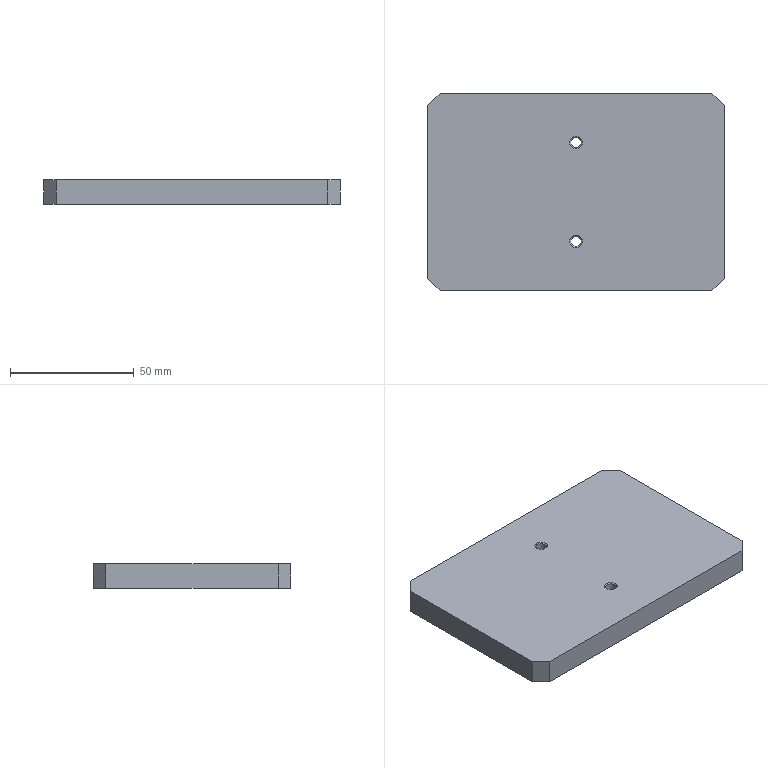Part | SolidWorks | features 3DProfileFeature 1, Chamfer 1, Extrusion 1, HoleWzd 1 | 1 solid | 18 faces | box 120 x 80 x 10 mm | volume 95220 mm3 | plane 10 | cone 4 | cylinder 4 | commonest cylinder face diameters 4.2 x4
STEP:
#1=CARTESIAN_POINT('',(-2.1,20.,9.575));
#2=VERTEX_POINT('',#1);
#3=CARTESIAN_POINT('',(2.1,20.,9.575));
#4=VERTEX_POINT('',#3);
#5=CARTESIAN_POINT('',(0.,20.,9.575));
#6=DIRECTION('',(0.,0.,1.));
#7=DIRECTION('',(1.,0.,0.));
#8=AXIS2_PLACEMENT_3D('',#5,#6,#7);
#9=CIRCLE('',#8,2.1);
#10=EDGE_CURVE('',#2,#4,#9,.T.);
#11=ORIENTED_EDGE('',*,*,#10,.F.);
#12=CARTESIAN_POINT('',(-2.525,20.,10.));
#13=VERTEX_POINT('',#12);
#14=CARTESIAN_POINT('',(-2.525,20.,10.));
#15=DIRECTION('',(-0.7071,0.,0.7071));
#16=VECTOR('',#15,1000.);
#17=LINE('',#14,#16);
#18=EDGE_CURVE('',#2,#13,#17,.T.);
#19=ORIENTED_EDGE('',*,*,#18,.T.);
#20=CARTESIAN_POINT('',(2.525,20.,10.));
#21=VERTEX_POINT('',#20);
#22=CARTESIAN_POINT('',(0.,20.,10.));
#23=DIRECTION('',(0.,0.,1.));
#24=DIRECTION('',(1.,0.,0.));
#25=AXIS2_PLACEMENT_3D('',#22,#23,#24);
#26=CIRCLE('',#25,2.525);
#27=EDGE_CURVE('',#13,#21,#26,.T.);
#28=ORIENTED_EDGE('',*,*,#27,.T.);
#29=CARTESIAN_POINT('',(2.525,20.,10.));
#30=DIRECTION('',(0.7071,0.,0.7071));
#31=VECTOR('',#30,1000.);
#32=LINE('',#29,#31);
#33=EDGE_CURVE('',#4,#21,#32,.T.);
#34=ORIENTED_EDGE('',*,*,#33,.F.);
#35=EDGE_LOOP('',(#11,#19,#28,#34));
#36=FACE_OUTER_BOUND('',#35,.T.);
#37=CARTESIAN_POINT('',(0.,20.,10.));
#38=DIRECTION('',(0.,0.,1.));
#39=DIRECTION('',(1.,0.,0.));
#40=AXIS2_PLACEMENT_3D('',#37,#38,#39);
#41=CONICAL_SURFACE('',#40,2.525,0.7854);
#42=ADVANCED_FACE('',(#36),#41,.F.);
#43=CARTESIAN_POINT('',(-2.1,20.,0.));
#44=VERTEX_POINT('',#43);
#45=CARTESIAN_POINT('',(2.1,20.,0.));
#46=VERTEX_POINT('',#45);
#47=CARTESIAN_POINT('',(0.,20.,0.));
#48=DIRECTION('',(0.,0.,1.));
#49=DIRECTION('',(1.,0.,0.));
#50=AXIS2_PLACEMENT_3D('',#47,#48,#49);
#51=CIRCLE('',#50,2.1);
#52=EDGE_CURVE('',#44,#46,#51,.T.);
#53=ORIENTED_EDGE('',*,*,#52,.F.);
#54=CARTESIAN_POINT('',(-2.1,20.,10.));
#55=DIRECTION('',(0.,0.,1.));
#56=VECTOR('',#55,1000.);
#57=LINE('',#54,#56);
#58=EDGE_CURVE('',#44,#2,#57,.T.);
#59=ORIENTED_EDGE('',*,*,#58,.T.);
#60=ORIENTED_EDGE('',*,*,#10,.T.);
#61=CARTESIAN_POINT('',(2.1,20.,10.));
#62=DIRECTION('',(0.,0.,1.));
#63=VECTOR('',#62,1000.);
#64=LINE('',#61,#63);
#65=EDGE_CURVE('',#46,#4,#64,.T.);
#66=ORIENTED_EDGE('',*,*,#65,.F.);
#67=EDGE_LOOP('',(#53,#59,#60,#66));
#68=FACE_OUTER_BOUND('',#67,.T.);
#69=CARTESIAN_POINT('',(0.,20.,10.));
#70=DIRECTION('',(0.,0.,1.));
#71=DIRECTION('',(1.,0.,0.));
#72=AXIS2_PLACEMENT_3D('',#69,#70,#71);
#73=CYLINDRICAL_SURFACE('',#72,2.1);
#74=ADVANCED_FACE('',(#68),#73,.F.);
#75=CARTESIAN_POINT('',(-2.1,-20.,9.575));
#76=VERTEX_POINT('',#75);
#77=CARTESIAN_POINT('',(2.1,-20.,9.575));
#78=VERTEX_POINT('',#77);
#79=CARTESIAN_POINT('',(0.,-20.,9.575));
#80=DIRECTION('',(0.,0.,1.));
#81=DIRECTION('',(1.,0.,0.));
#82=AXIS2_PLACEMENT_3D('',#79,#80,#81);
#83=CIRCLE('',#82,2.1);
#84=EDGE_CURVE('',#76,#78,#83,.T.);
#85=ORIENTED_EDGE('',*,*,#84,.F.);
#86=CARTESIAN_POINT('',(-2.525,-20.,10.));
#87=VERTEX_POINT('',#86);
#88=CARTESIAN_POINT('',(-2.525,-20.,10.));
#89=DIRECTION('',(-0.7071,0.,0.7071));
#90=VECTOR('',#89,1000.);
#91=LINE('',#88,#90);
#92=EDGE_CURVE('',#76,#87,#91,.T.);
#93=ORIENTED_EDGE('',*,*,#92,.T.);
#94=CARTESIAN_POINT('',(2.525,-20.,10.));
#95=VERTEX_POINT('',#94);
#96=CARTESIAN_POINT('',(0.,-20.,10.));
#97=DIRECTION('',(0.,0.,1.));
#98=DIRECTION('',(1.,0.,0.));
#99=AXIS2_PLACEMENT_3D('',#96,#97,#98);
#100=CIRCLE('',#99,2.525);
#101=EDGE_CURVE('',#87,#95,#100,.T.);
#102=ORIENTED_EDGE('',*,*,#101,.T.);
#103=CARTESIAN_POINT('',(2.525,-20.,10.));
#104=DIRECTION('',(0.7071,0.,0.7071));
#105=VECTOR('',#104,1000.);
#106=LINE('',#103,#105);
#107=EDGE_CURVE('',#78,#95,#106,.T.);
#108=ORIENTED_EDGE('',*,*,#107,.F.);
#109=EDGE_LOOP('',(#85,#93,#102,#108));
#110=FACE_OUTER_BOUND('',#109,.T.);
#111=CARTESIAN_POINT('',(0.,-20.,10.));
#112=DIRECTION('',(0.,0.,1.));
#113=DIRECTION('',(1.,0.,0.));
#114=AXIS2_PLACEMENT_3D('',#111,#112,#113);
#115=CONICAL_SURFACE('',#114,2.525,0.7854);
#116=ADVANCED_FACE('',(#110),#115,.F.);
#117=CARTESIAN_POINT('',(-2.1,-20.,0.));
#118=VERTEX_POINT('',#117);
#119=CARTESIAN_POINT('',(2.1,-20.,0.));
#120=VERTEX_POINT('',#119);
#121=CARTESIAN_POINT('',(0.,-20.,0.));
#122=DIRECTION('',(0.,0.,1.));
#123=DIRECTION('',(1.,0.,0.));
#124=AXIS2_PLACEMENT_3D('',#121,#122,#123);
#125=CIRCLE('',#124,2.1);
#126=EDGE_CURVE('',#118,#120,#125,.T.);
#127=ORIENTED_EDGE('',*,*,#126,.F.);
#128=CARTESIAN_POINT('',(-2.1,-20.,10.));
#129=DIRECTION('',(0.,0.,1.));
#130=VECTOR('',#129,1000.);
#131=LINE('',#128,#130);
#132=EDGE_CURVE('',#118,#76,#131,.T.);
#133=ORIENTED_EDGE('',*,*,#132,.T.);
#134=ORIENTED_EDGE('',*,*,#84,.T.);
#135=CARTESIAN_POINT('',(2.1,-20.,10.));
#136=DIRECTION('',(0.,0.,1.));
#137=VECTOR('',#136,1000.);
#138=LINE('',#135,#137);
#139=EDGE_CURVE('',#120,#78,#138,.T.);
#140=ORIENTED_EDGE('',*,*,#139,.F.);
#141=EDGE_LOOP('',(#127,#133,#134,#140));
#142=FACE_OUTER_BOUND('',#141,.T.);
#143=CARTESIAN_POINT('',(0.,-20.,10.));
#144=DIRECTION('',(0.,0.,1.));
#145=DIRECTION('',(1.,0.,0.));
#146=AXIS2_PLACEMENT_3D('',#143,#144,#145);
#147=CYLINDRICAL_SURFACE('',#146,2.1);
#148=ADVANCED_FACE('',(#142),#147,.F.);
#149=CARTESIAN_POINT('',(60.,-35.,10.));
#150=VERTEX_POINT('',#149);
#151=CARTESIAN_POINT('',(60.,35.,10.));
#152=VERTEX_POINT('',#151);
#153=CARTESIAN_POINT('',(60.,40.,10.));
#154=DIRECTION('',(0.,1.,0.));
#155=VECTOR('',#154,1000.);
#156=LINE('',#153,#155);
#157=EDGE_CURVE('',#150,#152,#156,.T.);
#158=ORIENTED_EDGE('',*,*,#157,.F.);
#159=CARTESIAN_POINT('',(60.,-35.,0.));
#160=VERTEX_POINT('',#159);
#161=CARTESIAN_POINT('',(60.,-35.,10.));
#162=DIRECTION('',(0.,0.,-1.));
#163=VECTOR('',#162,1000.);
#164=LINE('',#161,#163);
#165=EDGE_CURVE('',#150,#160,#164,.T.);
#166=ORIENTED_EDGE('',*,*,#165,.T.);
#167=CARTESIAN_POINT('',(60.,35.,0.));
#168=VERTEX_POINT('',#167);
#169=CARTESIAN_POINT('',(60.,40.,0.));
#170=DIRECTION('',(0.,1.,0.));
#171=VECTOR('',#170,1000.);
#172=LINE('',#169,#171);
#173=EDGE_CURVE('',#160,#168,#172,.T.);
#174=ORIENTED_EDGE('',*,*,#173,.T.);
#175=CARTESIAN_POINT('',(60.,35.,10.));
#176=DIRECTION('',(0.,0.,1.));
#177=VECTOR('',#176,1000.);
#178=LINE('',#175,#177);
#179=EDGE_CURVE('',#168,#152,#178,.T.);
#180=ORIENTED_EDGE('',*,*,#179,.T.);
#181=EDGE_LOOP('',(#158,#166,#174,#180));
#182=FACE_OUTER_BOUND('',#181,.T.);
#183=CARTESIAN_POINT('',(60.,40.,10.));
#184=DIRECTION('',(-1.,0.,0.));
#185=DIRECTION('',(0.,-1.,0.));
#186=AXIS2_PLACEMENT_3D('',#183,#184,#185);
#187=PLANE('',#186);
#188=ADVANCED_FACE('',(#182),#187,.F.);
#189=CARTESIAN_POINT('',(55.,40.,10.));
#190=VERTEX_POINT('',#189);
#191=CARTESIAN_POINT('',(-55.,40.,10.));
#192=VERTEX_POINT('',#191);
#193=CARTESIAN_POINT('',(-60.,40.,10.));
#194=DIRECTION('',(-1.,0.,0.));
#195=VECTOR('',#194,1000.);
#196=LINE('',#193,#195);
#197=EDGE_CURVE('',#190,#192,#196,.T.);
#198=ORIENTED_EDGE('',*,*,#197,.F.);
#199=CARTESIAN_POINT('',(55.,40.,0.));
#200=VERTEX_POINT('',#199);
#201=CARTESIAN_POINT('',(55.,40.,10.));
#202=DIRECTION('',(0.,0.,-1.));
#203=VECTOR('',#202,1000.);
#204=LINE('',#201,#203);
#205=EDGE_CURVE('',#190,#200,#204,.T.);
#206=ORIENTED_EDGE('',*,*,#205,.T.);
#207=CARTESIAN_POINT('',(-55.,40.,0.));
#208=VERTEX_POINT('',#207);
#209=CARTESIAN_POINT('',(-60.,40.,0.));
#210=DIRECTION('',(-1.,0.,0.));
#211=VECTOR('',#210,1000.);
#212=LINE('',#209,#211);
#213=EDGE_CURVE('',#200,#208,#212,.T.);
#214=ORIENTED_EDGE('',*,*,#213,.T.);
#215=CARTESIAN_POINT('',(-55.,40.,10.));
#216=DIRECTION('',(0.,0.,1.));
#217=VECTOR('',#216,1000.);
#218=LINE('',#215,#217);
#219=EDGE_CURVE('',#208,#192,#218,.T.);
#220=ORIENTED_EDGE('',*,*,#219,.T.);
#221=EDGE_LOOP('',(#198,#206,#214,#220));
#222=FACE_OUTER_BOUND('',#221,.T.);
#223=CARTESIAN_POINT('',(-60.,40.,10.));
#224=DIRECTION('',(0.,-1.,0.));
#225=DIRECTION('',(0.,0.,-1.));
#226=AXIS2_PLACEMENT_3D('',#223,#224,#225);
#227=PLANE('',#226);
#228=ADVANCED_FACE('',(#222),#227,.F.);
#229=CARTESIAN_POINT('',(-60.,35.,0.));
#230=VERTEX_POINT('',#229);
#231=CARTESIAN_POINT('',(-60.,-35.,0.));
#232=VERTEX_POINT('',#231);
#233=CARTESIAN_POINT('',(-60.,40.,0.));
#234=DIRECTION('',(0.,-1.,0.));
#235=VECTOR('',#234,1000.);
#236=LINE('',#233,#235);
#237=EDGE_CURVE('',#230,#232,#236,.T.);
#238=ORIENTED_EDGE('',*,*,#237,.T.);
#239=CARTESIAN_POINT('',(-60.,-35.,10.));
#240=VERTEX_POINT('',#239);
#241=CARTESIAN_POINT('',(-60.,-35.,10.));
#242=DIRECTION('',(0.,0.,1.));
#243=VECTOR('',#242,1000.);
#244=LINE('',#241,#243);
#245=EDGE_CURVE('',#232,#240,#244,.T.);
#246=ORIENTED_EDGE('',*,*,#245,.T.);
#247=CARTESIAN_POINT('',(-60.,35.,10.));
#248=VERTEX_POINT('',#247);
#249=CARTESIAN_POINT('',(-60.,40.,10.));
#250=DIRECTION('',(0.,-1.,0.));
#251=VECTOR('',#250,1000.);
#252=LINE('',#249,#251);
#253=EDGE_CURVE('',#248,#240,#252,.T.);
#254=ORIENTED_EDGE('',*,*,#253,.F.);
#255=CARTESIAN_POINT('',(-60.,35.,10.));
#256=DIRECTION('',(0.,0.,-1.));
#257=VECTOR('',#256,1000.);
#258=LINE('',#255,#257);
#259=EDGE_CURVE('',#248,#230,#258,.T.);
#260=ORIENTED_EDGE('',*,*,#259,.T.);
#261=EDGE_LOOP('',(#238,#246,#254,#260));
#262=FACE_OUTER_BOUND('',#261,.T.);
#263=CARTESIAN_POINT('',(-60.,40.,10.));
#264=DIRECTION('',(1.,0.,0.));
#265=DIRECTION('',(0.,0.,-1.));
#266=AXIS2_PLACEMENT_3D('',#263,#264,#265);
#267=PLANE('',#266);
#268=ADVANCED_FACE('',(#262),#267,.F.);
#269=CARTESIAN_POINT('',(-55.,-40.,0.));
#270=VERTEX_POINT('',#269);
#271=CARTESIAN_POINT('',(55.,-40.,0.));
#272=VERTEX_POINT('',#271);
#273=CARTESIAN_POINT('',(-60.,-40.,0.));
#274=DIRECTION('',(1.,0.,0.));
#275=VECTOR('',#274,1000.);
#276=LINE('',#273,#275);
#277=EDGE_CURVE('',#270,#272,#276,.T.);
#278=ORIENTED_EDGE('',*,*,#277,.T.);
#279=CARTESIAN_POINT('',(55.,-40.,10.));
#280=VERTEX_POINT('',#279);
#281=CARTESIAN_POINT('',(55.,-40.,10.));
#282=DIRECTION('',(0.,0.,1.));
#283=VECTOR('',#282,1000.);
#284=LINE('',#281,#283);
#285=EDGE_CURVE('',#272,#280,#284,.T.);
#286=ORIENTED_EDGE('',*,*,#285,.T.);
#287=CARTESIAN_POINT('',(-55.,-40.,10.));
#288=VERTEX_POINT('',#287);
#289=CARTESIAN_POINT('',(-60.,-40.,10.));
#290=DIRECTION('',(1.,0.,0.));
#291=VECTOR('',#290,1000.);
#292=LINE('',#289,#291);
#293=EDGE_CURVE('',#288,#280,#292,.T.);
#294=ORIENTED_EDGE('',*,*,#293,.F.);
#295=CARTESIAN_POINT('',(-55.,-40.,10.));
#296=DIRECTION('',(0.,0.,-1.));
#297=VECTOR('',#296,1000.);
#298=LINE('',#295,#297);
#299=EDGE_CURVE('',#288,#270,#298,.T.);
#300=ORIENTED_EDGE('',*,*,#299,.T.);
#301=EDGE_LOOP('',(#278,#286,#294,#300));
#302=FACE_OUTER_BOUND('',#301,.T.);
#303=CARTESIAN_POINT('',(-60.,-40.,10.));
#304=DIRECTION('',(0.,1.,0.));
#305=DIRECTION('',(0.,0.,1.));
#306=AXIS2_PLACEMENT_3D('',#303,#304,#305);
#307=PLANE('',#306);
#308=ADVANCED_FACE('',(#302),#307,.F.);
#309=CARTESIAN_POINT('',(0.,20.,10.));
#310=DIRECTION('',(0.,0.,1.));
#311=DIRECTION('',(1.,0.,0.));
#312=AXIS2_PLACEMENT_3D('',#309,#310,#311);
#313=CIRCLE('',#312,2.525);
#314=EDGE_CURVE('',#21,#13,#313,.T.);
#315=ORIENTED_EDGE('',*,*,#314,.F.);
#316=ORIENTED_EDGE('',*,*,#27,.F.);
#317=EDGE_LOOP('',(#315,#316));
#318=FACE_BOUND('',#317,.T.);
#319=CARTESIAN_POINT('',(0.,-20.,10.));
#320=DIRECTION('',(0.,0.,1.));
#321=DIRECTION('',(1.,0.,0.));
#322=AXIS2_PLACEMENT_3D('',#319,#320,#321);
#323=CIRCLE('',#322,2.525);
#324=EDGE_CURVE('',#95,#87,#323,.T.);
#325=ORIENTED_EDGE('',*,*,#324,.F.);
#326=ORIENTED_EDGE('',*,*,#101,.F.);
#327=EDGE_LOOP('',(#325,#326));
#328=FACE_BOUND('',#327,.T.);
#329=ORIENTED_EDGE('',*,*,#293,.T.);
#330=CARTESIAN_POINT('',(47.5,-47.5,10.));
#331=DIRECTION('',(0.7071,0.7071,0.));
#332=VECTOR('',#331,1000.);
#333=LINE('',#330,#332);
#334=EDGE_CURVE('',#280,#150,#333,.T.);
#335=ORIENTED_EDGE('',*,*,#334,.T.);
#336=ORIENTED_EDGE('',*,*,#157,.T.);
#337=CARTESIAN_POINT('',(47.5,47.5,10.));
#338=DIRECTION('',(-0.7071,0.7071,0.));
#339=VECTOR('',#338,1000.);
#340=LINE('',#337,#339);
#341=EDGE_CURVE('',#152,#190,#340,.T.);
#342=ORIENTED_EDGE('',*,*,#341,.T.);
#343=ORIENTED_EDGE('',*,*,#197,.T.);
#344=CARTESIAN_POINT('',(-47.5,47.5,10.));
#345=DIRECTION('',(-0.7071,-0.7071,0.));
#346=VECTOR('',#345,1000.);
#347=LINE('',#344,#346);
#348=EDGE_CURVE('',#192,#248,#347,.T.);
#349=ORIENTED_EDGE('',*,*,#348,.T.);
#350=ORIENTED_EDGE('',*,*,#253,.T.);
#351=CARTESIAN_POINT('',(-47.5,-47.5,10.));
#352=DIRECTION('',(0.7071,-0.7071,0.));
#353=VECTOR('',#352,1000.);
#354=LINE('',#351,#353);
#355=EDGE_CURVE('',#240,#288,#354,.T.);
#356=ORIENTED_EDGE('',*,*,#355,.T.);
#357=EDGE_LOOP('',(#329,#335,#336,#342,#343,#349,#350,#356));
#358=FACE_OUTER_BOUND('',#357,.T.);
#359=CARTESIAN_POINT('',(0.,0.,10.));
#360=DIRECTION('',(0.,0.,1.));
#361=DIRECTION('',(1.,0.,0.));
#362=AXIS2_PLACEMENT_3D('',#359,#360,#361);
#363=PLANE('',#362);
#364=ADVANCED_FACE('',(#318,#328,#358),#363,.T.);
#365=CARTESIAN_POINT('',(0.,20.,0.));
#366=DIRECTION('',(0.,0.,1.));
#367=DIRECTION('',(1.,0.,0.));
#368=AXIS2_PLACEMENT_3D('',#365,#366,#367);
#369=CIRCLE('',#368,2.1);
#370=EDGE_CURVE('',#46,#44,#369,.T.);
#371=ORIENTED_EDGE('',*,*,#370,.T.);
#372=ORIENTED_EDGE('',*,*,#52,.T.);
#373=EDGE_LOOP('',(#371,#372));
#374=FACE_BOUND('',#373,.T.);
#375=CARTESIAN_POINT('',(0.,-20.,0.));
#376=DIRECTION('',(0.,0.,1.));
#377=DIRECTION('',(1.,0.,0.));
#378=AXIS2_PLACEMENT_3D('',#375,#376,#377);
#379=CIRCLE('',#378,2.1);
#380=EDGE_CURVE('',#120,#118,#379,.T.);
#381=ORIENTED_EDGE('',*,*,#380,.T.);
#382=ORIENTED_EDGE('',*,*,#126,.T.);
#383=EDGE_LOOP('',(#381,#382));
#384=FACE_BOUND('',#383,.T.);
#385=ORIENTED_EDGE('',*,*,#173,.F.);
#386=CARTESIAN_POINT('',(60.,-35.,0.));
#387=DIRECTION('',(-0.7071,-0.7071,0.));
#388=VECTOR('',#387,1000.);
#389=LINE('',#386,#388);
#390=EDGE_CURVE('',#160,#272,#389,.T.);
#391=ORIENTED_EDGE('',*,*,#390,.T.);
#392=ORIENTED_EDGE('',*,*,#277,.F.);
#393=CARTESIAN_POINT('',(-55.,-40.,0.));
#394=DIRECTION('',(-0.7071,0.7071,0.));
#395=VECTOR('',#394,1000.);
#396=LINE('',#393,#395);
#397=EDGE_CURVE('',#270,#232,#396,.T.);
#398=ORIENTED_EDGE('',*,*,#397,.T.);
#399=ORIENTED_EDGE('',*,*,#237,.F.);
#400=CARTESIAN_POINT('',(-60.,35.,0.));
#401=DIRECTION('',(0.7071,0.7071,0.));
#402=VECTOR('',#401,1000.);
#403=LINE('',#400,#402);
#404=EDGE_CURVE('',#230,#208,#403,.T.);
#405=ORIENTED_EDGE('',*,*,#404,.T.);
#406=ORIENTED_EDGE('',*,*,#213,.F.);
#407=CARTESIAN_POINT('',(55.,40.,0.));
#408=DIRECTION('',(0.7071,-0.7071,0.));
#409=VECTOR('',#408,1000.);
#410=LINE('',#407,#409);
#411=EDGE_CURVE('',#200,#168,#410,.T.);
#412=ORIENTED_EDGE('',*,*,#411,.T.);
#413=EDGE_LOOP('',(#385,#391,#392,#398,#399,#405,#406,#412));
#414=FACE_OUTER_BOUND('',#413,.T.);
#415=CARTESIAN_POINT('',(0.,0.,0.));
#416=DIRECTION('',(0.,0.,1.));
#417=DIRECTION('',(1.,0.,0.));
#418=AXIS2_PLACEMENT_3D('',#415,#416,#417);
#419=PLANE('',#418);
#420=ADVANCED_FACE('',(#374,#384,#414),#419,.F.);
#421=ORIENTED_EDGE('',*,*,#334,.F.);
#422=ORIENTED_EDGE('',*,*,#285,.F.);
#423=ORIENTED_EDGE('',*,*,#390,.F.);
#424=ORIENTED_EDGE('',*,*,#165,.F.);
#425=EDGE_LOOP('',(#421,#422,#423,#424));
#426=FACE_OUTER_BOUND('',#425,.T.);
#427=CARTESIAN_POINT('',(60.,-35.,10.));
#428=DIRECTION('',(-0.7071,0.7071,0.));
#429=DIRECTION('',(0.,0.,-1.));
#430=AXIS2_PLACEMENT_3D('',#427,#428,#429);
#431=PLANE('',#430);
#432=ADVANCED_FACE('',(#426),#431,.F.);
#433=ORIENTED_EDGE('',*,*,#355,.F.);
#434=ORIENTED_EDGE('',*,*,#245,.F.);
#435=ORIENTED_EDGE('',*,*,#397,.F.);
#436=ORIENTED_EDGE('',*,*,#299,.F.);
#437=EDGE_LOOP('',(#433,#434,#435,#436));
#438=FACE_OUTER_BOUND('',#437,.T.);
#439=CARTESIAN_POINT('',(-55.,-40.,10.));
#440=DIRECTION('',(0.7071,0.7071,0.));
#441=DIRECTION('',(0.,0.,-1.));
#442=AXIS2_PLACEMENT_3D('',#439,#440,#441);
#443=PLANE('',#442);
#444=ADVANCED_FACE('',(#438),#443,.F.);
#445=ORIENTED_EDGE('',*,*,#341,.F.);
#446=ORIENTED_EDGE('',*,*,#179,.F.);
#447=ORIENTED_EDGE('',*,*,#411,.F.);
#448=ORIENTED_EDGE('',*,*,#205,.F.);
#449=EDGE_LOOP('',(#445,#446,#447,#448));
#450=FACE_OUTER_BOUND('',#449,.T.);
#451=CARTESIAN_POINT('',(55.,40.,10.));
#452=DIRECTION('',(-0.7071,-0.7071,0.));
#453=DIRECTION('',(0.,0.,-1.));
#454=AXIS2_PLACEMENT_3D('',#451,#452,#453);
#455=PLANE('',#454);
#456=ADVANCED_FACE('',(#450),#455,.F.);
#457=ORIENTED_EDGE('',*,*,#348,.F.);
#458=ORIENTED_EDGE('',*,*,#219,.F.);
#459=ORIENTED_EDGE('',*,*,#404,.F.);
#460=ORIENTED_EDGE('',*,*,#259,.F.);
#461=EDGE_LOOP('',(#457,#458,#459,#460));
#462=FACE_OUTER_BOUND('',#461,.T.);
#463=CARTESIAN_POINT('',(-60.,35.,10.));
#464=DIRECTION('',(0.7071,-0.7071,0.));
#465=DIRECTION('',(0.,0.,-1.));
#466=AXIS2_PLACEMENT_3D('',#463,#464,#465);
#467=PLANE('',#466);
#468=ADVANCED_FACE('',(#462),#467,.F.);
#469=ORIENTED_EDGE('',*,*,#132,.F.);
#470=ORIENTED_EDGE('',*,*,#380,.F.);
#471=ORIENTED_EDGE('',*,*,#139,.T.);
#472=CARTESIAN_POINT('',(0.,-20.,9.575));
#473=DIRECTION('',(0.,0.,1.));
#474=DIRECTION('',(1.,0.,0.));
#475=AXIS2_PLACEMENT_3D('',#472,#473,#474);
#476=CIRCLE('',#475,2.1);
#477=EDGE_CURVE('',#78,#76,#476,.T.);
#478=ORIENTED_EDGE('',*,*,#477,.T.);
#479=EDGE_LOOP('',(#469,#470,#471,#478));
#480=FACE_OUTER_BOUND('',#479,.T.);
#481=CARTESIAN_POINT('',(0.,-20.,10.));
#482=DIRECTION('',(0.,0.,1.));
#483=DIRECTION('',(1.,0.,0.));
#484=AXIS2_PLACEMENT_3D('',#481,#482,#483);
#485=CYLINDRICAL_SURFACE('',#484,2.1);
#486=ADVANCED_FACE('',(#480),#485,.F.);
#487=ORIENTED_EDGE('',*,*,#92,.F.);
#488=ORIENTED_EDGE('',*,*,#477,.F.);
#489=ORIENTED_EDGE('',*,*,#107,.T.);
#490=ORIENTED_EDGE('',*,*,#324,.T.);
#491=EDGE_LOOP('',(#487,#488,#489,#490));
#492=FACE_OUTER_BOUND('',#491,.T.);
#493=CARTESIAN_POINT('',(0.,-20.,10.));
#494=DIRECTION('',(0.,0.,1.));
#495=DIRECTION('',(1.,0.,0.));
#496=AXIS2_PLACEMENT_3D('',#493,#494,#495);
#497=CONICAL_SURFACE('',#496,2.525,0.7854);
#498=ADVANCED_FACE('',(#492),#497,.F.);
#499=ORIENTED_EDGE('',*,*,#58,.F.);
#500=ORIENTED_EDGE('',*,*,#370,.F.);
#501=ORIENTED_EDGE('',*,*,#65,.T.);
#502=CARTESIAN_POINT('',(0.,20.,9.575));
#503=DIRECTION('',(0.,0.,1.));
#504=DIRECTION('',(1.,0.,0.));
#505=AXIS2_PLACEMENT_3D('',#502,#503,#504);
#506=CIRCLE('',#505,2.1);
#507=EDGE_CURVE('',#4,#2,#506,.T.);
#508=ORIENTED_EDGE('',*,*,#507,.T.);
#509=EDGE_LOOP('',(#499,#500,#501,#508));
#510=FACE_OUTER_BOUND('',#509,.T.);
#511=CARTESIAN_POINT('',(0.,20.,10.));
#512=DIRECTION('',(0.,0.,1.));
#513=DIRECTION('',(1.,0.,0.));
#514=AXIS2_PLACEMENT_3D('',#511,#512,#513);
#515=CYLINDRICAL_SURFACE('',#514,2.1);
#516=ADVANCED_FACE('',(#510),#515,.F.);
#517=ORIENTED_EDGE('',*,*,#18,.F.);
#518=ORIENTED_EDGE('',*,*,#507,.F.);
#519=ORIENTED_EDGE('',*,*,#33,.T.);
#520=ORIENTED_EDGE('',*,*,#314,.T.);
#521=EDGE_LOOP('',(#517,#518,#519,#520));
#522=FACE_OUTER_BOUND('',#521,.T.);
#523=CARTESIAN_POINT('',(0.,20.,10.));
#524=DIRECTION('',(0.,0.,1.));
#525=DIRECTION('',(1.,0.,0.));
#526=AXIS2_PLACEMENT_3D('',#523,#524,#525);
#527=CONICAL_SURFACE('',#526,2.525,0.7854);
#528=ADVANCED_FACE('',(#522),#527,.F.);
#529=CLOSED_SHELL('',(#42,#74,#116,#148,#188,#228,#268,#308,#364,#420,#432,#444,#456,#468,#486,#498,#516,#528));
#530=MANIFOLD_SOLID_BREP('',#529);
#531=CARTESIAN_POINT('',(0.,0.,0.));
#532=DIRECTION('',(0.,0.,1.));
#533=DIRECTION('',(1.,0.,0.));
#534=AXIS2_PLACEMENT_3D('',#531,#532,#533);
#535=(LENGTH_UNIT()NAMED_UNIT(*)SI_UNIT(.MILLI.,.METRE.));
#536=UNCERTAINTY_MEASURE_WITH_UNIT(LENGTH_MEASURE(0.00001),#535,'','');
#537=(NAMED_UNIT(*)PLANE_ANGLE_UNIT()SI_UNIT($,.RADIAN.));
#538=(NAMED_UNIT(*)SI_UNIT($,.STERADIAN.)SOLID_ANGLE_UNIT());
#539=(GEOMETRIC_REPRESENTATION_CONTEXT(3)GLOBAL_UNCERTAINTY_ASSIGNED_CONTEXT((#536))GLOBAL_UNIT_ASSIGNED_CONTEXT((#535,#537,#538))REPRESENTATION_CONTEXT('',''));
#540=ADVANCED_BREP_SHAPE_REPRESENTATION('',(#530,#534),#539);